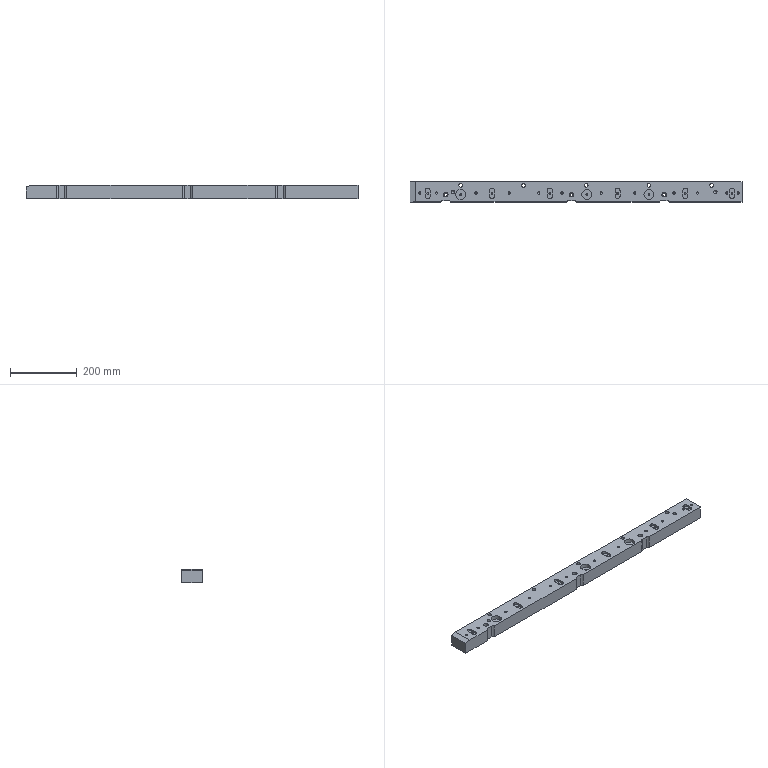Part | NX | features 22 2 | 1 solid | 130 faces | box 995 x 60 x 40 mm | volume 2260039 mm3 | cylinder 64 | plane 43 | cone 23 | commonest cylinder face diameters 6.8 x12 15 x12 5.2 x9 14 x9 6 x6 11 x5